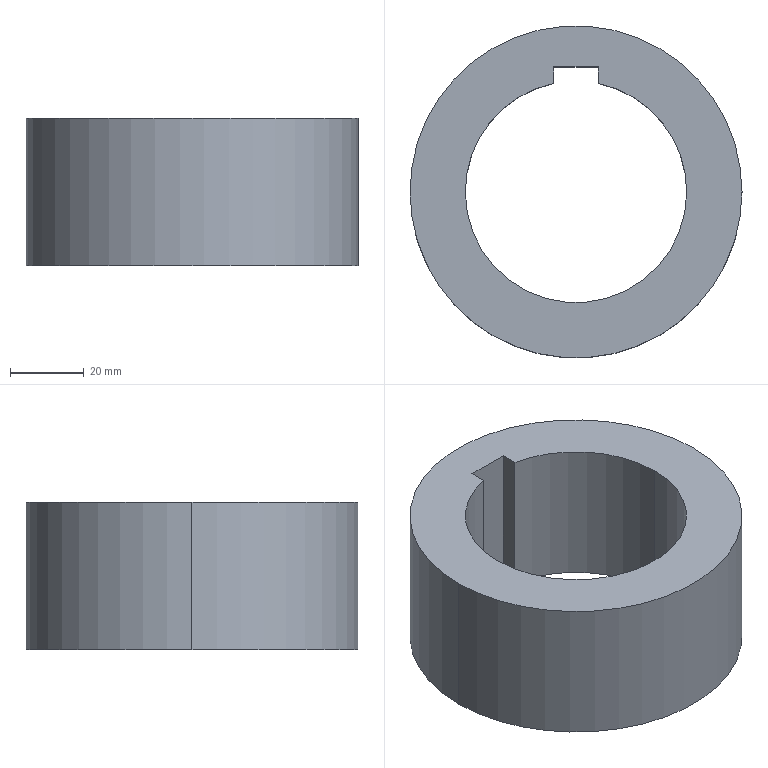Part | STEP file | 40 bushing | 1 solid | 10 faces | box 90 x 90 x 40 mm | volume 139406 mm3 | cylinder 5 | plane 5 | commonest cylinder face diameters 60 x3 90 x2
STEP:
#1=CARTESIAN_POINT('',(0.,0.,0.));
#2=DIRECTION('',(0.,0.,1.));
#3=DIRECTION('',(1.,0.,0.));
#4=AXIS2_PLACEMENT_3D('',#1,#2,#3);
#5=CARTESIAN_POINT('',(-30.,0.,20.));
#6=VERTEX_POINT('',#5);
#7=CARTESIAN_POINT('',(-30.,0.,-20.));
#8=VERTEX_POINT('',#7);
#9=CARTESIAN_POINT('',(-30.,0.,20.));
#10=DIRECTION('',(0.,0.,-1.));
#11=VECTOR('',#10,1.);
#12=LINE('',#9,#11);
#13=CARTESIAN_POINT('',(0.,0.,20.));
#14=DIRECTION('',(0.,0.,-1.));
#15=DIRECTION('',(-1.,0.,0.));
#16=AXIS2_PLACEMENT_3D('',#13,#14,#15);
#17=CYLINDRICAL_SURFACE('',#16,30.);
#18=CARTESIAN_POINT('',(6.283,0.));
#19=DIRECTION('',(0.,1.));
#20=VECTOR('',#19,1.);
#21=LINE('',#18,#20);
#22=(GEOMETRIC_REPRESENTATION_CONTEXT(2)PARAMETRIC_REPRESENTATION_CONTEXT()REPRESENTATION_CONTEXT('',''));
#23=DEFINITIONAL_REPRESENTATION('',(#21),#22);
#24=PCURVE('',#17,#23);
#25=CARTESIAN_POINT('',(0.,0.,20.));
#26=DIRECTION('',(0.,0.,-1.));
#27=DIRECTION('',(-1.,0.,0.));
#28=AXIS2_PLACEMENT_3D('',#25,#26,#27);
#29=CYLINDRICAL_SURFACE('',#28,30.);
#30=CARTESIAN_POINT('',(0.,0.));
#31=DIRECTION('',(0.,1.));
#32=VECTOR('',#31,1.);
#33=LINE('',#30,#32);
#34=(GEOMETRIC_REPRESENTATION_CONTEXT(2)PARAMETRIC_REPRESENTATION_CONTEXT()REPRESENTATION_CONTEXT('',''));
#35=DEFINITIONAL_REPRESENTATION('',(#33),#34);
#36=PCURVE('',#29,#35);
#37=SURFACE_CURVE('',#12,(#24,#36),.PCURVE_S1.);
#38=EDGE_CURVE('',#6,#8,#37,.T.);
#39=ORIENTED_EDGE('',*,*,#38,.T.);
#40=CARTESIAN_POINT('',(30.,0.,-20.));
#41=VERTEX_POINT('',#40);
#42=CARTESIAN_POINT('',(0.,0.,-20.));
#43=DIRECTION('',(0.,0.,1.));
#44=DIRECTION('',(1.,0.,0.));
#45=AXIS2_PLACEMENT_3D('',#42,#43,#44);
#46=CIRCLE('',#45,30.);
#47=CARTESIAN_POINT('',(9.425,40.));
#48=DIRECTION('',(-1.,0.));
#49=VECTOR('',#48,1.);
#50=LINE('',#47,#49);
#51=(GEOMETRIC_REPRESENTATION_CONTEXT(2)PARAMETRIC_REPRESENTATION_CONTEXT()REPRESENTATION_CONTEXT('',''));
#52=DEFINITIONAL_REPRESENTATION('',(#50),#51);
#53=PCURVE('',#17,#52);
#54=CARTESIAN_POINT('',(0.,0.,-20.));
#55=DIRECTION('',(0.,0.,1.));
#56=DIRECTION('',(1.,0.,0.));
#57=AXIS2_PLACEMENT_3D('',#54,#55,#56);
#58=PLANE('',#57);
#59=CARTESIAN_POINT('',(0.,0.));
#60=DIRECTION('',(1.,0.));
#61=AXIS2_PLACEMENT_2D('',#59,#60);
#62=CIRCLE('',#61,30.);
#63=(GEOMETRIC_REPRESENTATION_CONTEXT(2)PARAMETRIC_REPRESENTATION_CONTEXT()REPRESENTATION_CONTEXT('',''));
#64=DEFINITIONAL_REPRESENTATION('',(#62),#63);
#65=PCURVE('',#58,#64);
#66=SURFACE_CURVE('',#46,(#53,#65),.PCURVE_S1.);
#67=EDGE_CURVE('',#8,#41,#66,.T.);
#68=ORIENTED_EDGE('',*,*,#67,.T.);
#69=CARTESIAN_POINT('',(30.,0.,20.));
#70=VERTEX_POINT('',#69);
#71=CARTESIAN_POINT('',(30.,0.,20.));
#72=DIRECTION('',(0.,0.,-1.));
#73=VECTOR('',#72,1.);
#74=LINE('',#71,#73);
#75=CARTESIAN_POINT('',(3.142,0.));
#76=DIRECTION('',(0.,1.));
#77=VECTOR('',#76,1.);
#78=LINE('',#75,#77);
#79=(GEOMETRIC_REPRESENTATION_CONTEXT(2)PARAMETRIC_REPRESENTATION_CONTEXT()REPRESENTATION_CONTEXT('',''));
#80=DEFINITIONAL_REPRESENTATION('',(#78),#79);
#81=PCURVE('',#17,#80);
#82=CARTESIAN_POINT('',(0.,0.,20.));
#83=DIRECTION('',(0.,0.,-1.));
#84=DIRECTION('',(-1.,0.,0.));
#85=AXIS2_PLACEMENT_3D('',#82,#83,#84);
#86=CYLINDRICAL_SURFACE('',#85,30.);
#87=CARTESIAN_POINT('',(3.142,0.));
#88=DIRECTION('',(0.,1.));
#89=VECTOR('',#88,1.);
#90=LINE('',#87,#89);
#91=(GEOMETRIC_REPRESENTATION_CONTEXT(2)PARAMETRIC_REPRESENTATION_CONTEXT()REPRESENTATION_CONTEXT('',''));
#92=DEFINITIONAL_REPRESENTATION('',(#90),#91);
#93=PCURVE('',#86,#92);
#94=SURFACE_CURVE('',#74,(#81,#93),.PCURVE_S1.);
#95=EDGE_CURVE('',#70,#41,#94,.T.);
#96=ORIENTED_EDGE('',*,*,#95,.F.);
#97=CARTESIAN_POINT('',(0.,0.,20.));
#98=DIRECTION('',(0.,0.,1.));
#99=DIRECTION('',(1.,0.,0.));
#100=AXIS2_PLACEMENT_3D('',#97,#98,#99);
#101=CIRCLE('',#100,30.);
#102=CARTESIAN_POINT('',(9.425,0.));
#103=DIRECTION('',(-1.,0.));
#104=VECTOR('',#103,1.);
#105=LINE('',#102,#104);
#106=(GEOMETRIC_REPRESENTATION_CONTEXT(2)PARAMETRIC_REPRESENTATION_CONTEXT()REPRESENTATION_CONTEXT('',''));
#107=DEFINITIONAL_REPRESENTATION('',(#105),#106);
#108=PCURVE('',#17,#107);
#109=CARTESIAN_POINT('',(0.,0.,20.));
#110=DIRECTION('',(0.,0.,1.));
#111=DIRECTION('',(1.,0.,0.));
#112=AXIS2_PLACEMENT_3D('',#109,#110,#111);
#113=PLANE('',#112);
#114=CARTESIAN_POINT('',(0.,0.));
#115=DIRECTION('',(1.,0.));
#116=AXIS2_PLACEMENT_2D('',#114,#115);
#117=CIRCLE('',#116,30.);
#118=(GEOMETRIC_REPRESENTATION_CONTEXT(2)PARAMETRIC_REPRESENTATION_CONTEXT()REPRESENTATION_CONTEXT('',''));
#119=DEFINITIONAL_REPRESENTATION('',(#117),#118);
#120=PCURVE('',#113,#119);
#121=SURFACE_CURVE('',#101,(#108,#120),.PCURVE_S1.);
#122=EDGE_CURVE('',#6,#70,#121,.T.);
#123=ORIENTED_EDGE('',*,*,#122,.F.);
#124=EDGE_LOOP('',(#39,#68,#96,#123));
#125=FACE_BOUND('',#124,.F.);
#126=ADVANCED_FACE('',(#125),#17,.F.);
#127=CARTESIAN_POINT('',(-6.,29.394,20.));
#128=VERTEX_POINT('',#127);
#129=CARTESIAN_POINT('',(-6.,29.394,-20.));
#130=VERTEX_POINT('',#129);
#131=CARTESIAN_POINT('',(-6.,29.394,20.));
#132=DIRECTION('',(0.,0.,-1.));
#133=VECTOR('',#132,1.);
#134=LINE('',#131,#133);
#135=CARTESIAN_POINT('',(1.369,0.));
#136=DIRECTION('',(0.,1.));
#137=VECTOR('',#136,1.);
#138=LINE('',#135,#137);
#139=(GEOMETRIC_REPRESENTATION_CONTEXT(2)PARAMETRIC_REPRESENTATION_CONTEXT()REPRESENTATION_CONTEXT('',''));
#140=DEFINITIONAL_REPRESENTATION('',(#138),#139);
#141=PCURVE('',#29,#140);
#142=CARTESIAN_POINT('',(-6.,33.894,20.));
#143=DIRECTION('',(1.,0.,0.));
#144=DIRECTION('',(0.,1.,0.));
#145=AXIS2_PLACEMENT_3D('',#142,#143,#144);
#146=PLANE('',#145);
#147=CARTESIAN_POINT('',(-4.5,0.));
#148=DIRECTION('',(0.,-1.));
#149=VECTOR('',#148,1.);
#150=LINE('',#147,#149);
#151=(GEOMETRIC_REPRESENTATION_CONTEXT(2)PARAMETRIC_REPRESENTATION_CONTEXT()REPRESENTATION_CONTEXT('',''));
#152=DEFINITIONAL_REPRESENTATION('',(#150),#151);
#153=PCURVE('',#146,#152);
#154=SURFACE_CURVE('',#134,(#141,#153),.PCURVE_S1.);
#155=EDGE_CURVE('',#128,#130,#154,.T.);
#156=ORIENTED_EDGE('',*,*,#155,.T.);
#157=CARTESIAN_POINT('',(0.,0.,-20.));
#158=DIRECTION('',(0.,0.,1.));
#159=DIRECTION('',(1.,0.,0.));
#160=AXIS2_PLACEMENT_3D('',#157,#158,#159);
#161=CIRCLE('',#160,30.);
#162=CARTESIAN_POINT('',(3.142,40.));
#163=DIRECTION('',(-1.,0.));
#164=VECTOR('',#163,1.);
#165=LINE('',#162,#164);
#166=(GEOMETRIC_REPRESENTATION_CONTEXT(2)PARAMETRIC_REPRESENTATION_CONTEXT()REPRESENTATION_CONTEXT('',''));
#167=DEFINITIONAL_REPRESENTATION('',(#165),#166);
#168=PCURVE('',#29,#167);
#169=CARTESIAN_POINT('',(0.,0.));
#170=DIRECTION('',(1.,0.));
#171=AXIS2_PLACEMENT_2D('',#169,#170);
#172=CIRCLE('',#171,30.);
#173=(GEOMETRIC_REPRESENTATION_CONTEXT(2)PARAMETRIC_REPRESENTATION_CONTEXT()REPRESENTATION_CONTEXT('',''));
#174=DEFINITIONAL_REPRESENTATION('',(#172),#173);
#175=PCURVE('',#58,#174);
#176=SURFACE_CURVE('',#161,(#168,#175),.PCURVE_S1.);
#177=EDGE_CURVE('',#130,#8,#176,.T.);
#178=ORIENTED_EDGE('',*,*,#177,.T.);
#179=ORIENTED_EDGE('',*,*,#38,.F.);
#180=CARTESIAN_POINT('',(0.,0.,20.));
#181=DIRECTION('',(0.,0.,1.));
#182=DIRECTION('',(1.,0.,0.));
#183=AXIS2_PLACEMENT_3D('',#180,#181,#182);
#184=CIRCLE('',#183,30.);
#185=CARTESIAN_POINT('',(3.142,0.));
#186=DIRECTION('',(-1.,0.));
#187=VECTOR('',#186,1.);
#188=LINE('',#185,#187);
#189=(GEOMETRIC_REPRESENTATION_CONTEXT(2)PARAMETRIC_REPRESENTATION_CONTEXT()REPRESENTATION_CONTEXT('',''));
#190=DEFINITIONAL_REPRESENTATION('',(#188),#189);
#191=PCURVE('',#29,#190);
#192=CARTESIAN_POINT('',(0.,0.));
#193=DIRECTION('',(1.,0.));
#194=AXIS2_PLACEMENT_2D('',#192,#193);
#195=CIRCLE('',#194,30.);
#196=(GEOMETRIC_REPRESENTATION_CONTEXT(2)PARAMETRIC_REPRESENTATION_CONTEXT()REPRESENTATION_CONTEXT('',''));
#197=DEFINITIONAL_REPRESENTATION('',(#195),#196);
#198=PCURVE('',#113,#197);
#199=SURFACE_CURVE('',#184,(#191,#198),.PCURVE_S1.);
#200=EDGE_CURVE('',#128,#6,#199,.T.);
#201=ORIENTED_EDGE('',*,*,#200,.F.);
#202=EDGE_LOOP('',(#156,#178,#179,#201));
#203=FACE_BOUND('',#202,.F.);
#204=ADVANCED_FACE('',(#203),#29,.F.);
#205=CARTESIAN_POINT('',(45.,0.,20.));
#206=VERTEX_POINT('',#205);
#207=CARTESIAN_POINT('',(-45.,0.,20.));
#208=VERTEX_POINT('',#207);
#209=CARTESIAN_POINT('',(0.,0.,20.));
#210=DIRECTION('',(0.,0.,1.));
#211=DIRECTION('',(1.,0.,0.));
#212=AXIS2_PLACEMENT_3D('',#209,#210,#211);
#213=CIRCLE('',#212,45.);
#214=CARTESIAN_POINT('',(0.,0.,20.));
#215=DIRECTION('',(0.,0.,-1.));
#216=DIRECTION('',(-1.,0.,0.));
#217=AXIS2_PLACEMENT_3D('',#214,#215,#216);
#218=CYLINDRICAL_SURFACE('',#217,45.);
#219=CARTESIAN_POINT('',(3.142,0.));
#220=DIRECTION('',(-1.,0.));
#221=VECTOR('',#220,1.);
#222=LINE('',#219,#221);
#223=(GEOMETRIC_REPRESENTATION_CONTEXT(2)PARAMETRIC_REPRESENTATION_CONTEXT()REPRESENTATION_CONTEXT('',''));
#224=DEFINITIONAL_REPRESENTATION('',(#222),#223);
#225=PCURVE('',#218,#224);
#226=CARTESIAN_POINT('',(0.,0.));
#227=DIRECTION('',(1.,0.));
#228=AXIS2_PLACEMENT_2D('',#226,#227);
#229=CIRCLE('',#228,45.);
#230=(GEOMETRIC_REPRESENTATION_CONTEXT(2)PARAMETRIC_REPRESENTATION_CONTEXT()REPRESENTATION_CONTEXT('',''));
#231=DEFINITIONAL_REPRESENTATION('',(#229),#230);
#232=PCURVE('',#113,#231);
#233=SURFACE_CURVE('',#213,(#225,#232),.PCURVE_S1.);
#234=EDGE_CURVE('',#206,#208,#233,.T.);
#235=ORIENTED_EDGE('',*,*,#234,.F.);
#236=CARTESIAN_POINT('',(45.,0.,-20.));
#237=VERTEX_POINT('',#236);
#238=CARTESIAN_POINT('',(45.,0.,20.));
#239=DIRECTION('',(0.,0.,-1.));
#240=VECTOR('',#239,1.);
#241=LINE('',#238,#240);
#242=CARTESIAN_POINT('',(3.142,0.));
#243=DIRECTION('',(0.,1.));
#244=VECTOR('',#243,1.);
#245=LINE('',#242,#244);
#246=(GEOMETRIC_REPRESENTATION_CONTEXT(2)PARAMETRIC_REPRESENTATION_CONTEXT()REPRESENTATION_CONTEXT('',''));
#247=DEFINITIONAL_REPRESENTATION('',(#245),#246);
#248=PCURVE('',#218,#247);
#249=CARTESIAN_POINT('',(0.,0.,20.));
#250=DIRECTION('',(0.,0.,-1.));
#251=DIRECTION('',(-1.,0.,0.));
#252=AXIS2_PLACEMENT_3D('',#249,#250,#251);
#253=CYLINDRICAL_SURFACE('',#252,45.);
#254=CARTESIAN_POINT('',(3.142,0.));
#255=DIRECTION('',(0.,1.));
#256=VECTOR('',#255,1.);
#257=LINE('',#254,#256);
#258=(GEOMETRIC_REPRESENTATION_CONTEXT(2)PARAMETRIC_REPRESENTATION_CONTEXT()REPRESENTATION_CONTEXT('',''));
#259=DEFINITIONAL_REPRESENTATION('',(#257),#258);
#260=PCURVE('',#253,#259);
#261=SURFACE_CURVE('',#241,(#248,#260),.PCURVE_S1.);
#262=EDGE_CURVE('',#206,#237,#261,.T.);
#263=ORIENTED_EDGE('',*,*,#262,.T.);
#264=CARTESIAN_POINT('',(-45.,0.,-20.));
#265=VERTEX_POINT('',#264);
#266=CARTESIAN_POINT('',(0.,0.,-20.));
#267=DIRECTION('',(0.,0.,1.));
#268=DIRECTION('',(1.,0.,0.));
#269=AXIS2_PLACEMENT_3D('',#266,#267,#268);
#270=CIRCLE('',#269,45.);
#271=CARTESIAN_POINT('',(3.142,40.));
#272=DIRECTION('',(-1.,0.));
#273=VECTOR('',#272,1.);
#274=LINE('',#271,#273);
#275=(GEOMETRIC_REPRESENTATION_CONTEXT(2)PARAMETRIC_REPRESENTATION_CONTEXT()REPRESENTATION_CONTEXT('',''));
#276=DEFINITIONAL_REPRESENTATION('',(#274),#275);
#277=PCURVE('',#218,#276);
#278=CARTESIAN_POINT('',(0.,0.));
#279=DIRECTION('',(1.,0.));
#280=AXIS2_PLACEMENT_2D('',#278,#279);
#281=CIRCLE('',#280,45.);
#282=(GEOMETRIC_REPRESENTATION_CONTEXT(2)PARAMETRIC_REPRESENTATION_CONTEXT()REPRESENTATION_CONTEXT('',''));
#283=DEFINITIONAL_REPRESENTATION('',(#281),#282);
#284=PCURVE('',#58,#283);
#285=SURFACE_CURVE('',#270,(#277,#284),.PCURVE_S1.);
#286=EDGE_CURVE('',#237,#265,#285,.T.);
#287=ORIENTED_EDGE('',*,*,#286,.T.);
#288=CARTESIAN_POINT('',(-45.,0.,20.));
#289=DIRECTION('',(0.,0.,-1.));
#290=VECTOR('',#289,1.);
#291=LINE('',#288,#290);
#292=CARTESIAN_POINT('',(0.,0.));
#293=DIRECTION('',(0.,1.));
#294=VECTOR('',#293,1.);
#295=LINE('',#292,#294);
#296=(GEOMETRIC_REPRESENTATION_CONTEXT(2)PARAMETRIC_REPRESENTATION_CONTEXT()REPRESENTATION_CONTEXT('',''));
#297=DEFINITIONAL_REPRESENTATION('',(#295),#296);
#298=PCURVE('',#218,#297);
#299=CARTESIAN_POINT('',(6.283,0.));
#300=DIRECTION('',(0.,1.));
#301=VECTOR('',#300,1.);
#302=LINE('',#299,#301);
#303=(GEOMETRIC_REPRESENTATION_CONTEXT(2)PARAMETRIC_REPRESENTATION_CONTEXT()REPRESENTATION_CONTEXT('',''));
#304=DEFINITIONAL_REPRESENTATION('',(#302),#303);
#305=PCURVE('',#253,#304);
#306=SURFACE_CURVE('',#291,(#298,#305),.PCURVE_S1.);
#307=EDGE_CURVE('',#208,#265,#306,.T.);
#308=ORIENTED_EDGE('',*,*,#307,.F.);
#309=EDGE_LOOP('',(#235,#263,#287,#308));
#310=FACE_BOUND('',#309,.T.);
#311=ADVANCED_FACE('',(#310),#218,.T.);
#312=CARTESIAN_POINT('',(0.,0.,20.));
#313=DIRECTION('',(0.,0.,1.));
#314=DIRECTION('',(1.,0.,0.));
#315=AXIS2_PLACEMENT_3D('',#312,#313,#314);
#316=CIRCLE('',#315,45.);
#317=CARTESIAN_POINT('',(0.,0.));
#318=DIRECTION('',(1.,0.));
#319=AXIS2_PLACEMENT_2D('',#317,#318);
#320=CIRCLE('',#319,45.);
#321=(GEOMETRIC_REPRESENTATION_CONTEXT(2)PARAMETRIC_REPRESENTATION_CONTEXT()REPRESENTATION_CONTEXT('',''));
#322=DEFINITIONAL_REPRESENTATION('',(#320),#321);
#323=PCURVE('',#113,#322);
#324=CARTESIAN_POINT('',(9.425,0.));
#325=DIRECTION('',(-1.,0.));
#326=VECTOR('',#325,1.);
#327=LINE('',#324,#326);
#328=(GEOMETRIC_REPRESENTATION_CONTEXT(2)PARAMETRIC_REPRESENTATION_CONTEXT()REPRESENTATION_CONTEXT('',''));
#329=DEFINITIONAL_REPRESENTATION('',(#327),#328);
#330=PCURVE('',#253,#329);
#331=SURFACE_CURVE('',#316,(#323,#330),.PCURVE_S1.);
#332=EDGE_CURVE('',#208,#206,#331,.T.);
#333=ORIENTED_EDGE('',*,*,#332,.T.);
#334=ORIENTED_EDGE('',*,*,#234,.T.);
#335=EDGE_LOOP('',(#333,#334));
#336=FACE_BOUND('',#335,.T.);
#337=CARTESIAN_POINT('',(6.,29.394,20.));
#338=VERTEX_POINT('',#337);
#339=CARTESIAN_POINT('',(6.,33.894,20.));
#340=VERTEX_POINT('',#339);
#341=CARTESIAN_POINT('',(6.,33.894,20.));
#342=DIRECTION('',(0.,1.,0.));
#343=VECTOR('',#342,1.);
#344=LINE('',#341,#343);
#345=CARTESIAN_POINT('',(6.,33.894));
#346=DIRECTION('',(0.,1.));
#347=VECTOR('',#346,1.);
#348=LINE('',#345,#347);
#349=(GEOMETRIC_REPRESENTATION_CONTEXT(2)PARAMETRIC_REPRESENTATION_CONTEXT()REPRESENTATION_CONTEXT('',''));
#350=DEFINITIONAL_REPRESENTATION('',(#348),#349);
#351=PCURVE('',#113,#350);
#352=CARTESIAN_POINT('',(6.,33.894,20.));
#353=DIRECTION('',(-1.,0.,0.));
#354=DIRECTION('',(0.,-1.,0.));
#355=AXIS2_PLACEMENT_3D('',#352,#353,#354);
#356=PLANE('',#355);
#357=CARTESIAN_POINT('',(0.,0.));
#358=DIRECTION('',(-1.,0.));
#359=VECTOR('',#358,1.);
#360=LINE('',#357,#359);
#361=(GEOMETRIC_REPRESENTATION_CONTEXT(2)PARAMETRIC_REPRESENTATION_CONTEXT()REPRESENTATION_CONTEXT('',''));
#362=DEFINITIONAL_REPRESENTATION('',(#360),#361);
#363=PCURVE('',#356,#362);
#364=SURFACE_CURVE('',#344,(#351,#363),.PCURVE_S1.);
#365=EDGE_CURVE('',#338,#340,#364,.T.);
#366=ORIENTED_EDGE('',*,*,#365,.F.);
#367=CARTESIAN_POINT('',(0.,0.,20.));
#368=DIRECTION('',(0.,0.,1.));
#369=DIRECTION('',(1.,0.,0.));
#370=AXIS2_PLACEMENT_3D('',#367,#368,#369);
#371=CIRCLE('',#370,30.);
#372=CARTESIAN_POINT('',(0.,0.));
#373=DIRECTION('',(1.,0.));
#374=AXIS2_PLACEMENT_2D('',#372,#373);
#375=CIRCLE('',#374,30.);
#376=(GEOMETRIC_REPRESENTATION_CONTEXT(2)PARAMETRIC_REPRESENTATION_CONTEXT()REPRESENTATION_CONTEXT('',''));
#377=DEFINITIONAL_REPRESENTATION('',(#375),#376);
#378=PCURVE('',#113,#377);
#379=CARTESIAN_POINT('',(3.142,0.));
#380=DIRECTION('',(-1.,0.));
#381=VECTOR('',#380,1.);
#382=LINE('',#379,#381);
#383=(GEOMETRIC_REPRESENTATION_CONTEXT(2)PARAMETRIC_REPRESENTATION_CONTEXT()REPRESENTATION_CONTEXT('',''));
#384=DEFINITIONAL_REPRESENTATION('',(#382),#383);
#385=PCURVE('',#86,#384);
#386=SURFACE_CURVE('',#371,(#378,#385),.PCURVE_S1.);
#387=EDGE_CURVE('',#70,#338,#386,.T.);
#388=ORIENTED_EDGE('',*,*,#387,.F.);
#389=ORIENTED_EDGE('',*,*,#122,.F.);
#390=ORIENTED_EDGE('',*,*,#200,.F.);
#391=CARTESIAN_POINT('',(-6.,33.894,20.));
#392=VERTEX_POINT('',#391);
#393=CARTESIAN_POINT('',(-6.,33.894,20.));
#394=DIRECTION('',(0.,-1.,0.));
#395=VECTOR('',#394,1.);
#396=LINE('',#393,#395);
#397=CARTESIAN_POINT('',(-6.,33.894));
#398=DIRECTION('',(0.,-1.));
#399=VECTOR('',#398,1.);
#400=LINE('',#397,#399);
#401=(GEOMETRIC_REPRESENTATION_CONTEXT(2)PARAMETRIC_REPRESENTATION_CONTEXT()REPRESENTATION_CONTEXT('',''));
#402=DEFINITIONAL_REPRESENTATION('',(#400),#401);
#403=PCURVE('',#113,#402);
#404=CARTESIAN_POINT('',(0.,0.));
#405=DIRECTION('',(-1.,0.));
#406=VECTOR('',#405,1.);
#407=LINE('',#404,#406);
#408=(GEOMETRIC_REPRESENTATION_CONTEXT(2)PARAMETRIC_REPRESENTATION_CONTEXT()REPRESENTATION_CONTEXT('',''));
#409=DEFINITIONAL_REPRESENTATION('',(#407),#408);
#410=PCURVE('',#146,#409);
#411=SURFACE_CURVE('',#396,(#403,#410),.PCURVE_S1.);
#412=EDGE_CURVE('',#392,#128,#411,.T.);
#413=ORIENTED_EDGE('',*,*,#412,.F.);
#414=CARTESIAN_POINT('',(-6.,33.894,20.));
#415=DIRECTION('',(-1.,0.,0.));
#416=VECTOR('',#415,1.);
#417=LINE('',#414,#416);
#418=CARTESIAN_POINT('',(-6.,33.894));
#419=DIRECTION('',(-1.,0.));
#420=VECTOR('',#419,1.);
#421=LINE('',#418,#420);
#422=(GEOMETRIC_REPRESENTATION_CONTEXT(2)PARAMETRIC_REPRESENTATION_CONTEXT()REPRESENTATION_CONTEXT('',''));
#423=DEFINITIONAL_REPRESENTATION('',(#421),#422);
#424=PCURVE('',#113,#423);
#425=CARTESIAN_POINT('',(-6.,33.894,20.));
#426=DIRECTION('',(0.,-1.,0.));
#427=DIRECTION('',(0.,0.,-1.));
#428=AXIS2_PLACEMENT_3D('',#425,#426,#427);
#429=PLANE('',#428);
#430=CARTESIAN_POINT('',(0.,0.));
#431=DIRECTION('',(0.,-1.));
#432=VECTOR('',#431,1.);
#433=LINE('',#430,#432);
#434=(GEOMETRIC_REPRESENTATION_CONTEXT(2)PARAMETRIC_REPRESENTATION_CONTEXT()REPRESENTATION_CONTEXT('',''));
#435=DEFINITIONAL_REPRESENTATION('',(#433),#434);
#436=PCURVE('',#429,#435);
#437=SURFACE_CURVE('',#417,(#424,#436),.PCURVE_S1.);
#438=EDGE_CURVE('',#340,#392,#437,.T.);
#439=ORIENTED_EDGE('',*,*,#438,.F.);
#440=EDGE_LOOP('',(#366,#388,#389,#390,#413,#439));
#441=FACE_BOUND('',#440,.T.);
#442=ADVANCED_FACE('',(#336,#441),#113,.T.);
#443=CARTESIAN_POINT('',(0.,0.,-20.));
#444=DIRECTION('',(0.,0.,1.));
#445=DIRECTION('',(1.,0.,0.));
#446=AXIS2_PLACEMENT_3D('',#443,#444,#445);
#447=CIRCLE('',#446,45.);
#448=CARTESIAN_POINT('',(0.,0.));
#449=DIRECTION('',(1.,0.));
#450=AXIS2_PLACEMENT_2D('',#448,#449);
#451=CIRCLE('',#450,45.);
#452=(GEOMETRIC_REPRESENTATION_CONTEXT(2)PARAMETRIC_REPRESENTATION_CONTEXT()REPRESENTATION_CONTEXT('',''));
#453=DEFINITIONAL_REPRESENTATION('',(#451),#452);
#454=PCURVE('',#58,#453);
#455=CARTESIAN_POINT('',(9.425,40.));
#456=DIRECTION('',(-1.,0.));
#457=VECTOR('',#456,1.);
#458=LINE('',#455,#457);
#459=(GEOMETRIC_REPRESENTATION_CONTEXT(2)PARAMETRIC_REPRESENTATION_CONTEXT()REPRESENTATION_CONTEXT('',''));
#460=DEFINITIONAL_REPRESENTATION('',(#458),#459);
#461=PCURVE('',#253,#460);
#462=SURFACE_CURVE('',#447,(#454,#461),.PCURVE_S1.);
#463=EDGE_CURVE('',#265,#237,#462,.T.);
#464=ORIENTED_EDGE('',*,*,#463,.F.);
#465=ORIENTED_EDGE('',*,*,#286,.F.);
#466=EDGE_LOOP('',(#464,#465));
#467=FACE_BOUND('',#466,.T.);
#468=ORIENTED_EDGE('',*,*,#177,.T.);
#469=ORIENTED_EDGE('',*,*,#67,.T.);
#470=CARTESIAN_POINT('',(6.,29.394,-20.));
#471=VERTEX_POINT('',#470);
#472=CARTESIAN_POINT('',(0.,0.,-20.));
#473=DIRECTION('',(0.,0.,1.));
#474=DIRECTION('',(1.,0.,0.));
#475=AXIS2_PLACEMENT_3D('',#472,#473,#474);
#476=CIRCLE('',#475,30.);
#477=CARTESIAN_POINT('',(0.,0.));
#478=DIRECTION('',(1.,0.));
#479=AXIS2_PLACEMENT_2D('',#477,#478);
#480=CIRCLE('',#479,30.);
#481=(GEOMETRIC_REPRESENTATION_CONTEXT(2)PARAMETRIC_REPRESENTATION_CONTEXT()REPRESENTATION_CONTEXT('',''));
#482=DEFINITIONAL_REPRESENTATION('',(#480),#481);
#483=PCURVE('',#58,#482);
#484=CARTESIAN_POINT('',(3.142,40.));
#485=DIRECTION('',(-1.,0.));
#486=VECTOR('',#485,1.);
#487=LINE('',#484,#486);
#488=(GEOMETRIC_REPRESENTATION_CONTEXT(2)PARAMETRIC_REPRESENTATION_CONTEXT()REPRESENTATION_CONTEXT('',''));
#489=DEFINITIONAL_REPRESENTATION('',(#487),#488);
#490=PCURVE('',#86,#489);
#491=SURFACE_CURVE('',#476,(#483,#490),.PCURVE_S1.);
#492=EDGE_CURVE('',#41,#471,#491,.T.);
#493=ORIENTED_EDGE('',*,*,#492,.T.);
#494=CARTESIAN_POINT('',(6.,33.894,-20.));
#495=VERTEX_POINT('',#494);
#496=CARTESIAN_POINT('',(6.,33.894,-20.));
#497=DIRECTION('',(0.,1.,0.));
#498=VECTOR('',#497,1.);
#499=LINE('',#496,#498);
#500=CARTESIAN_POINT('',(6.,33.894));
#501=DIRECTION('',(0.,1.));
#502=VECTOR('',#501,1.);
#503=LINE('',#500,#502);
#504=(GEOMETRIC_REPRESENTATION_CONTEXT(2)PARAMETRIC_REPRESENTATION_CONTEXT()REPRESENTATION_CONTEXT('',''));
#505=DEFINITIONAL_REPRESENTATION('',(#503),#504);
#506=PCURVE('',#58,#505);
#507=CARTESIAN_POINT('',(0.,-40.));
#508=DIRECTION('',(-1.,0.));
#509=VECTOR('',#508,1.);
#510=LINE('',#507,#509);
#511=(GEOMETRIC_REPRESENTATION_CONTEXT(2)PARAMETRIC_REPRESENTATION_CONTEXT()REPRESENTATION_CONTEXT('',''));
#512=DEFINITIONAL_REPRESENTATION('',(#510),#511);
#513=PCURVE('',#356,#512);
#514=SURFACE_CURVE('',#499,(#506,#513),.PCURVE_S1.);
#515=EDGE_CURVE('',#471,#495,#514,.T.);
#516=ORIENTED_EDGE('',*,*,#515,.T.);
#517=CARTESIAN_POINT('',(-6.,33.894,-20.));
#518=VERTEX_POINT('',#517);
#519=CARTESIAN_POINT('',(-6.,33.894,-20.));
#520=DIRECTION('',(-1.,0.,0.));
#521=VECTOR('',#520,1.);
#522=LINE('',#519,#521);
#523=CARTESIAN_POINT('',(-6.,33.894));
#524=DIRECTION('',(-1.,0.));
#525=VECTOR('',#524,1.);
#526=LINE('',#523,#525);
#527=(GEOMETRIC_REPRESENTATION_CONTEXT(2)PARAMETRIC_REPRESENTATION_CONTEXT()REPRESENTATION_CONTEXT('',''));
#528=DEFINITIONAL_REPRESENTATION('',(#526),#527);
#529=PCURVE('',#58,#528);
#530=CARTESIAN_POINT('',(40.,0.));
#531=DIRECTION('',(0.,-1.));
#532=VECTOR('',#531,1.);
#533=LINE('',#530,#532);
#534=(GEOMETRIC_REPRESENTATION_CONTEXT(2)PARAMETRIC_REPRESENTATION_CONTEXT()REPRESENTATION_CONTEXT('',''));
#535=DEFINITIONAL_REPRESENTATION('',(#533),#534);
#536=PCURVE('',#429,#535);
#537=SURFACE_CURVE('',#522,(#529,#536),.PCURVE_S1.);
#538=EDGE_CURVE('',#495,#518,#537,.T.);
#539=ORIENTED_EDGE('',*,*,#538,.T.);
#540=CARTESIAN_POINT('',(-6.,33.894,-20.));
#541=DIRECTION('',(0.,-1.,0.));
#542=VECTOR('',#541,1.);
#543=LINE('',#540,#542);
#544=CARTESIAN_POINT('',(-6.,33.894));
#545=DIRECTION('',(0.,-1.));
#546=VECTOR('',#545,1.);
#547=LINE('',#544,#546);
#548=(GEOMETRIC_REPRESENTATION_CONTEXT(2)PARAMETRIC_REPRESENTATION_CONTEXT()REPRESENTATION_CONTEXT('',''));
#549=DEFINITIONAL_REPRESENTATION('',(#547),#548);
#550=PCURVE('',#58,#549);
#551=CARTESIAN_POINT('',(0.,-40.));
#552=DIRECTION('',(-1.,0.));
#553=VECTOR('',#552,1.);
#554=LINE('',#551,#553);
#555=(GEOMETRIC_REPRESENTATION_CONTEXT(2)PARAMETRIC_REPRESENTATION_CONTEXT()REPRESENTATION_CONTEXT('',''));
#556=DEFINITIONAL_REPRESENTATION('',(#554),#555);
#557=PCURVE('',#146,#556);
#558=SURFACE_CURVE('',#543,(#550,#557),.PCURVE_S1.);
#559=EDGE_CURVE('',#518,#130,#558,.T.);
#560=ORIENTED_EDGE('',*,*,#559,.T.);
#561=EDGE_LOOP('',(#468,#469,#493,#516,#539,#560));
#562=FACE_BOUND('',#561,.T.);
#563=ADVANCED_FACE('',(#467,#562),#58,.F.);
#564=ORIENTED_EDGE('',*,*,#262,.F.);
#565=ORIENTED_EDGE('',*,*,#332,.F.);
#566=ORIENTED_EDGE('',*,*,#307,.T.);
#567=ORIENTED_EDGE('',*,*,#463,.T.);
#568=EDGE_LOOP('',(#564,#565,#566,#567));
#569=FACE_BOUND('',#568,.T.);
#570=ADVANCED_FACE('',(#569),#253,.T.);
#571=ORIENTED_EDGE('',*,*,#492,.T.);
#572=CARTESIAN_POINT('',(6.,29.394,20.));
#573=DIRECTION('',(0.,0.,-1.));
#574=VECTOR('',#573,1.);
#575=LINE('',#572,#574);
#576=CARTESIAN_POINT('',(1.772,0.));
#577=DIRECTION('',(0.,1.));
#578=VECTOR('',#577,1.);
#579=LINE('',#576,#578);
#580=(GEOMETRIC_REPRESENTATION_CONTEXT(2)PARAMETRIC_REPRESENTATION_CONTEXT()REPRESENTATION_CONTEXT('',''));
#581=DEFINITIONAL_REPRESENTATION('',(#579),#580);
#582=PCURVE('',#86,#581);
#583=CARTESIAN_POINT('',(4.5,0.));
#584=DIRECTION('',(0.,-1.));
#585=VECTOR('',#584,1.);
#586=LINE('',#583,#585);
#587=(GEOMETRIC_REPRESENTATION_CONTEXT(2)PARAMETRIC_REPRESENTATION_CONTEXT()REPRESENTATION_CONTEXT('',''));
#588=DEFINITIONAL_REPRESENTATION('',(#586),#587);
#589=PCURVE('',#356,#588);
#590=SURFACE_CURVE('',#575,(#582,#589),.PCURVE_S1.);
#591=EDGE_CURVE('',#338,#471,#590,.T.);
#592=ORIENTED_EDGE('',*,*,#591,.F.);
#593=ORIENTED_EDGE('',*,*,#387,.F.);
#594=ORIENTED_EDGE('',*,*,#95,.T.);
#595=EDGE_LOOP('',(#571,#592,#593,#594));
#596=FACE_BOUND('',#595,.F.);
#597=ADVANCED_FACE('',(#596),#86,.F.);
#598=ORIENTED_EDGE('',*,*,#515,.F.);
#599=ORIENTED_EDGE('',*,*,#591,.F.);
#600=ORIENTED_EDGE('',*,*,#365,.T.);
#601=CARTESIAN_POINT('',(6.,33.894,20.));
#602=DIRECTION('',(0.,0.,-1.));
#603=VECTOR('',#602,1.);
#604=LINE('',#601,#603);
#605=CARTESIAN_POINT('',(0.,0.));
#606=DIRECTION('',(0.,-1.));
#607=VECTOR('',#606,1.);
#608=LINE('',#605,#607);
#609=(GEOMETRIC_REPRESENTATION_CONTEXT(2)PARAMETRIC_REPRESENTATION_CONTEXT()REPRESENTATION_CONTEXT('',''));
#610=DEFINITIONAL_REPRESENTATION('',(#608),#609);
#611=PCURVE('',#356,#610);
#612=CARTESIAN_POINT('',(0.,12.));
#613=DIRECTION('',(1.,0.));
#614=VECTOR('',#613,1.);
#615=LINE('',#612,#614);
#616=(GEOMETRIC_REPRESENTATION_CONTEXT(2)PARAMETRIC_REPRESENTATION_CONTEXT()REPRESENTATION_CONTEXT('',''));
#617=DEFINITIONAL_REPRESENTATION('',(#615),#616);
#618=PCURVE('',#429,#617);
#619=SURFACE_CURVE('',#604,(#611,#618),.PCURVE_S1.);
#620=EDGE_CURVE('',#340,#495,#619,.T.);
#621=ORIENTED_EDGE('',*,*,#620,.T.);
#622=EDGE_LOOP('',(#598,#599,#600,#621));
#623=FACE_BOUND('',#622,.T.);
#624=ADVANCED_FACE('',(#623),#356,.T.);
#625=ORIENTED_EDGE('',*,*,#538,.F.);
#626=ORIENTED_EDGE('',*,*,#620,.F.);
#627=ORIENTED_EDGE('',*,*,#438,.T.);
#628=CARTESIAN_POINT('',(-6.,33.894,20.));
#629=DIRECTION('',(0.,0.,-1.));
#630=VECTOR('',#629,1.);
#631=LINE('',#628,#630);
#632=CARTESIAN_POINT('',(0.,0.));
#633=DIRECTION('',(1.,0.));
#634=VECTOR('',#633,1.);
#635=LINE('',#632,#634);
#636=(GEOMETRIC_REPRESENTATION_CONTEXT(2)PARAMETRIC_REPRESENTATION_CONTEXT()REPRESENTATION_CONTEXT('',''));
#637=DEFINITIONAL_REPRESENTATION('',(#635),#636);
#638=PCURVE('',#429,#637);
#639=CARTESIAN_POINT('',(0.,0.));
#640=DIRECTION('',(0.,-1.));
#641=VECTOR('',#640,1.);
#642=LINE('',#639,#641);
#643=(GEOMETRIC_REPRESENTATION_CONTEXT(2)PARAMETRIC_REPRESENTATION_CONTEXT()REPRESENTATION_CONTEXT('',''));
#644=DEFINITIONAL_REPRESENTATION('',(#642),#643);
#645=PCURVE('',#146,#644);
#646=SURFACE_CURVE('',#631,(#638,#645),.PCURVE_S1.);
#647=EDGE_CURVE('',#392,#518,#646,.T.);
#648=ORIENTED_EDGE('',*,*,#647,.T.);
#649=EDGE_LOOP('',(#625,#626,#627,#648));
#650=FACE_BOUND('',#649,.T.);
#651=ADVANCED_FACE('',(#650),#429,.T.);
#652=ORIENTED_EDGE('',*,*,#559,.F.);
#653=ORIENTED_EDGE('',*,*,#647,.F.);
#654=ORIENTED_EDGE('',*,*,#412,.T.);
#655=ORIENTED_EDGE('',*,*,#155,.T.);
#656=EDGE_LOOP('',(#652,#653,#654,#655));
#657=FACE_BOUND('',#656,.T.);
#658=ADVANCED_FACE('',(#657),#146,.T.);
#659=CLOSED_SHELL('',(#126,#204,#311,#442,#563,#570,#597,#624,#651,#658));
#660=MANIFOLD_SOLID_BREP('',#659);
#661=(LENGTH_UNIT()NAMED_UNIT(*)SI_UNIT(.MILLI.,.METRE.));
#662=UNCERTAINTY_MEASURE_WITH_UNIT(LENGTH_MEASURE(0.0000001),#661,'','');
#663=(NAMED_UNIT(*)PLANE_ANGLE_UNIT()SI_UNIT($,.RADIAN.));
#664=(NAMED_UNIT(*)SI_UNIT($,.STERADIAN.)SOLID_ANGLE_UNIT());
#665=(GEOMETRIC_REPRESENTATION_CONTEXT(3)GLOBAL_UNCERTAINTY_ASSIGNED_CONTEXT((#662))GLOBAL_UNIT_ASSIGNED_CONTEXT((#661,#663,#664))REPRESENTATION_CONTEXT('',''));
#666=ADVANCED_BREP_SHAPE_REPRESENTATION('',(#4,#660),#665);